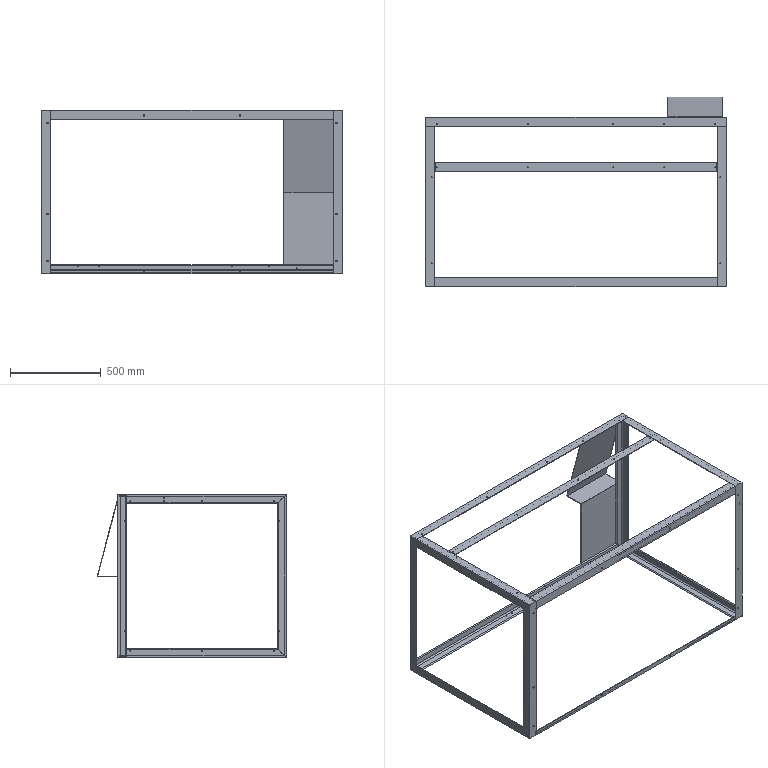Part | STEP file | OP10-002_upper frame(Default_As Machined_) | 14 solids | 302 faces | box 1650 x 1042 x 900 mm | volume 8540478 mm3 | cylinder 194 | plane 108 | commonest cylinder face diameters 5 x92 10 x47 16 x24 8 x22 4.2 x8 7 x1